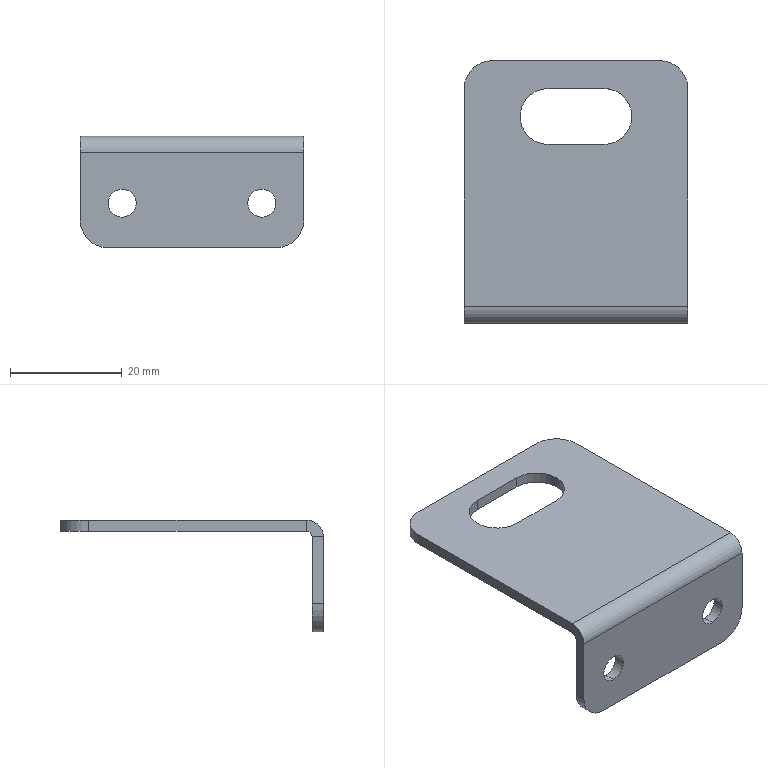Part | SolidWorks | features BaseBody 1 | 1 solid | 27 faces | box 40 x 47 x 20 mm | volume 4653 mm3 | plane 14 | cylinder 13 | commonest cylinder face diameters 10 x7 5 x4 2 x1 6 x1
STEP:
#1=CARTESIAN_POINT('',(-20.,-23.5,-15.));
#2=VERTEX_POINT('',#1);
#3=CARTESIAN_POINT('',(-15.,-23.5,-20.));
#4=VERTEX_POINT('',#3);
#5=CARTESIAN_POINT('',(-15.,-23.5,-15.));
#6=DIRECTION('',(0.,-1.,0.));
#7=DIRECTION('',(0.,0.,1.));
#8=AXIS2_PLACEMENT_3D('',#5,#6,#7);
#9=CIRCLE('',#8,5.);
#10=EDGE_CURVE('',#2,#4,#9,.T.);
#11=ORIENTED_EDGE('',*,*,#10,.F.);
#12=CARTESIAN_POINT('',(-20.,-21.5,-15.));
#13=VERTEX_POINT('',#12);
#14=CARTESIAN_POINT('',(-20.,-23.5,-15.));
#15=DIRECTION('',(0.,-1.,0.));
#16=VECTOR('',#15,1000.);
#17=LINE('',#14,#16);
#18=EDGE_CURVE('',#13,#2,#17,.T.);
#19=ORIENTED_EDGE('',*,*,#18,.F.);
#20=CARTESIAN_POINT('',(-15.,-21.5,-20.));
#21=VERTEX_POINT('',#20);
#22=CARTESIAN_POINT('',(-15.,-21.5,-15.));
#23=DIRECTION('',(0.,1.,0.));
#24=DIRECTION('',(0.,0.,1.));
#25=AXIS2_PLACEMENT_3D('',#22,#23,#24);
#26=CIRCLE('',#25,5.);
#27=EDGE_CURVE('',#21,#13,#26,.T.);
#28=ORIENTED_EDGE('',*,*,#27,.F.);
#29=CARTESIAN_POINT('',(-15.,-23.5,-20.));
#30=DIRECTION('',(0.,1.,0.));
#31=VECTOR('',#30,1000.);
#32=LINE('',#29,#31);
#33=EDGE_CURVE('',#4,#21,#32,.T.);
#34=ORIENTED_EDGE('',*,*,#33,.F.);
#35=EDGE_LOOP('',(#11,#19,#28,#34));
#36=FACE_OUTER_BOUND('',#35,.T.);
#37=CARTESIAN_POINT('',(-15.,-23.5,-15.));
#38=DIRECTION('',(0.,1.,0.));
#39=DIRECTION('',(0.,0.,1.));
#40=AXIS2_PLACEMENT_3D('',#37,#38,#39);
#41=CYLINDRICAL_SURFACE('',#40,5.);
#42=ADVANCED_FACE('',(#36),#41,.T.);
#43=CARTESIAN_POINT('',(15.,-23.5,-20.));
#44=VERTEX_POINT('',#43);
#45=CARTESIAN_POINT('',(20.,-23.5,-15.));
#46=VERTEX_POINT('',#45);
#47=CARTESIAN_POINT('',(15.,-23.5,-15.));
#48=DIRECTION('',(0.,-1.,0.));
#49=DIRECTION('',(0.,0.,1.));
#50=AXIS2_PLACEMENT_3D('',#47,#48,#49);
#51=CIRCLE('',#50,5.);
#52=EDGE_CURVE('',#44,#46,#51,.T.);
#53=ORIENTED_EDGE('',*,*,#52,.F.);
#54=CARTESIAN_POINT('',(15.,-21.5,-20.));
#55=VERTEX_POINT('',#54);
#56=CARTESIAN_POINT('',(15.,-23.5,-20.));
#57=DIRECTION('',(0.,-1.,0.));
#58=VECTOR('',#57,1000.);
#59=LINE('',#56,#58);
#60=EDGE_CURVE('',#55,#44,#59,.T.);
#61=ORIENTED_EDGE('',*,*,#60,.F.);
#62=CARTESIAN_POINT('',(20.,-21.5,-15.));
#63=VERTEX_POINT('',#62);
#64=CARTESIAN_POINT('',(15.,-21.5,-15.));
#65=DIRECTION('',(0.,1.,0.));
#66=DIRECTION('',(0.,0.,1.));
#67=AXIS2_PLACEMENT_3D('',#64,#65,#66);
#68=CIRCLE('',#67,5.);
#69=EDGE_CURVE('',#63,#55,#68,.T.);
#70=ORIENTED_EDGE('',*,*,#69,.F.);
#71=CARTESIAN_POINT('',(20.,-23.5,-15.));
#72=DIRECTION('',(0.,1.,0.));
#73=VECTOR('',#72,1000.);
#74=LINE('',#71,#73);
#75=EDGE_CURVE('',#46,#63,#74,.T.);
#76=ORIENTED_EDGE('',*,*,#75,.F.);
#77=EDGE_LOOP('',(#53,#61,#70,#76));
#78=FACE_OUTER_BOUND('',#77,.T.);
#79=CARTESIAN_POINT('',(15.,-23.5,-15.));
#80=DIRECTION('',(0.,1.,0.));
#81=DIRECTION('',(0.,0.,1.));
#82=AXIS2_PLACEMENT_3D('',#79,#80,#81);
#83=CYLINDRICAL_SURFACE('',#82,5.);
#84=ADVANCED_FACE('',(#78),#83,.T.);
#85=CARTESIAN_POINT('',(15.,23.5,-2.));
#86=VERTEX_POINT('',#85);
#87=CARTESIAN_POINT('',(20.,18.5,-2.));
#88=VERTEX_POINT('',#87);
#89=CARTESIAN_POINT('',(15.,18.5,-2.));
#90=DIRECTION('',(0.,0.,-1.));
#91=DIRECTION('',(-1.,0.,0.));
#92=AXIS2_PLACEMENT_3D('',#89,#90,#91);
#93=CIRCLE('',#92,5.);
#94=EDGE_CURVE('',#86,#88,#93,.T.);
#95=ORIENTED_EDGE('',*,*,#94,.F.);
#96=CARTESIAN_POINT('',(15.,23.5,0.));
#97=VERTEX_POINT('',#96);
#98=CARTESIAN_POINT('',(15.,23.5,-2.));
#99=DIRECTION('',(0.,0.,-1.));
#100=VECTOR('',#99,1000.);
#101=LINE('',#98,#100);
#102=EDGE_CURVE('',#97,#86,#101,.T.);
#103=ORIENTED_EDGE('',*,*,#102,.F.);
#104=CARTESIAN_POINT('',(20.,18.5,0.));
#105=VERTEX_POINT('',#104);
#106=CARTESIAN_POINT('',(15.,18.5,0.));
#107=DIRECTION('',(0.,0.,1.));
#108=DIRECTION('',(-1.,0.,0.));
#109=AXIS2_PLACEMENT_3D('',#106,#107,#108);
#110=CIRCLE('',#109,5.);
#111=EDGE_CURVE('',#105,#97,#110,.T.);
#112=ORIENTED_EDGE('',*,*,#111,.F.);
#113=CARTESIAN_POINT('',(20.,18.5,-2.));
#114=DIRECTION('',(0.,0.,1.));
#115=VECTOR('',#114,1000.);
#116=LINE('',#113,#115);
#117=EDGE_CURVE('',#88,#105,#116,.T.);
#118=ORIENTED_EDGE('',*,*,#117,.F.);
#119=EDGE_LOOP('',(#95,#103,#112,#118));
#120=FACE_OUTER_BOUND('',#119,.T.);
#121=CARTESIAN_POINT('',(15.,18.5,-2.));
#122=DIRECTION('',(0.,0.,1.));
#123=DIRECTION('',(1.,0.,0.));
#124=AXIS2_PLACEMENT_3D('',#121,#122,#123);
#125=CYLINDRICAL_SURFACE('',#124,5.);
#126=ADVANCED_FACE('',(#120),#125,.T.);
#127=CARTESIAN_POINT('',(-20.,18.5,-2.));
#128=VERTEX_POINT('',#127);
#129=CARTESIAN_POINT('',(-15.,23.5,-2.));
#130=VERTEX_POINT('',#129);
#131=CARTESIAN_POINT('',(-15.,18.5,-2.));
#132=DIRECTION('',(0.,0.,-1.));
#133=DIRECTION('',(-1.,0.,0.));
#134=AXIS2_PLACEMENT_3D('',#131,#132,#133);
#135=CIRCLE('',#134,5.);
#136=EDGE_CURVE('',#128,#130,#135,.T.);
#137=ORIENTED_EDGE('',*,*,#136,.F.);
#138=CARTESIAN_POINT('',(-20.,18.5,0.));
#139=VERTEX_POINT('',#138);
#140=CARTESIAN_POINT('',(-20.,18.5,-2.));
#141=DIRECTION('',(0.,0.,-1.));
#142=VECTOR('',#141,1000.);
#143=LINE('',#140,#142);
#144=EDGE_CURVE('',#139,#128,#143,.T.);
#145=ORIENTED_EDGE('',*,*,#144,.F.);
#146=CARTESIAN_POINT('',(-15.,23.5,0.));
#147=VERTEX_POINT('',#146);
#148=CARTESIAN_POINT('',(-15.,18.5,0.));
#149=DIRECTION('',(0.,0.,1.));
#150=DIRECTION('',(-1.,0.,0.));
#151=AXIS2_PLACEMENT_3D('',#148,#149,#150);
#152=CIRCLE('',#151,5.);
#153=EDGE_CURVE('',#147,#139,#152,.T.);
#154=ORIENTED_EDGE('',*,*,#153,.F.);
#155=CARTESIAN_POINT('',(-15.,23.5,-2.));
#156=DIRECTION('',(0.,0.,1.));
#157=VECTOR('',#156,1000.);
#158=LINE('',#155,#157);
#159=EDGE_CURVE('',#130,#147,#158,.T.);
#160=ORIENTED_EDGE('',*,*,#159,.F.);
#161=EDGE_LOOP('',(#137,#145,#154,#160));
#162=FACE_OUTER_BOUND('',#161,.T.);
#163=CARTESIAN_POINT('',(-15.,18.5,-2.));
#164=DIRECTION('',(0.,0.,1.));
#165=DIRECTION('',(1.,0.,0.));
#166=AXIS2_PLACEMENT_3D('',#163,#164,#165);
#167=CYLINDRICAL_SURFACE('',#166,5.);
#168=ADVANCED_FACE('',(#162),#167,.T.);
#169=CARTESIAN_POINT('',(-12.5,-21.5,-9.5));
#170=VERTEX_POINT('',#169);
#171=CARTESIAN_POINT('',(-12.5,-23.5,-9.5));
#172=VERTEX_POINT('',#171);
#173=CARTESIAN_POINT('',(-12.5,-21.5,-9.5));
#174=DIRECTION('',(0.,-1.,0.));
#175=VECTOR('',#174,1000.);
#176=LINE('',#173,#175);
#177=EDGE_CURVE('',#170,#172,#176,.T.);
#178=ORIENTED_EDGE('',*,*,#177,.F.);
#179=CARTESIAN_POINT('',(-12.5,-21.5,-14.5));
#180=VERTEX_POINT('',#179);
#181=CARTESIAN_POINT('',(-12.5,-21.5,-12.));
#182=DIRECTION('',(0.,-1.,0.));
#183=DIRECTION('',(0.,0.,-1.));
#184=AXIS2_PLACEMENT_3D('',#181,#182,#183);
#185=CIRCLE('',#184,2.5);
#186=EDGE_CURVE('',#180,#170,#185,.T.);
#187=ORIENTED_EDGE('',*,*,#186,.F.);
#188=CARTESIAN_POINT('',(-12.5,-23.5,-14.5));
#189=VERTEX_POINT('',#188);
#190=CARTESIAN_POINT('',(-12.5,-21.5,-14.5));
#191=DIRECTION('',(0.,-1.,0.));
#192=VECTOR('',#191,1000.);
#193=LINE('',#190,#192);
#194=EDGE_CURVE('',#180,#189,#193,.T.);
#195=ORIENTED_EDGE('',*,*,#194,.T.);
#196=CARTESIAN_POINT('',(-12.5,-23.5,-12.));
#197=DIRECTION('',(0.,-1.,0.));
#198=DIRECTION('',(0.,0.,-1.));
#199=AXIS2_PLACEMENT_3D('',#196,#197,#198);
#200=CIRCLE('',#199,2.5);
#201=EDGE_CURVE('',#189,#172,#200,.T.);
#202=ORIENTED_EDGE('',*,*,#201,.T.);
#203=EDGE_LOOP('',(#178,#187,#195,#202));
#204=FACE_OUTER_BOUND('',#203,.T.);
#205=CARTESIAN_POINT('',(-12.5,-21.5,-12.));
#206=DIRECTION('',(0.,-1.,0.));
#207=DIRECTION('',(0.,0.,-1.));
#208=AXIS2_PLACEMENT_3D('',#205,#206,#207);
#209=CYLINDRICAL_SURFACE('',#208,2.5);
#210=ADVANCED_FACE('',(#204),#209,.F.);
#211=CARTESIAN_POINT('',(12.5,-21.5,-9.5));
#212=VERTEX_POINT('',#211);
#213=CARTESIAN_POINT('',(12.5,-23.5,-9.5));
#214=VERTEX_POINT('',#213);
#215=CARTESIAN_POINT('',(12.5,-21.5,-9.5));
#216=DIRECTION('',(0.,-1.,0.));
#217=VECTOR('',#216,1000.);
#218=LINE('',#215,#217);
#219=EDGE_CURVE('',#212,#214,#218,.T.);
#220=ORIENTED_EDGE('',*,*,#219,.F.);
#221=CARTESIAN_POINT('',(12.5,-21.5,-14.5));
#222=VERTEX_POINT('',#221);
#223=CARTESIAN_POINT('',(12.5,-21.5,-12.));
#224=DIRECTION('',(0.,-1.,0.));
#225=DIRECTION('',(0.,0.,1.));
#226=AXIS2_PLACEMENT_3D('',#223,#224,#225);
#227=CIRCLE('',#226,2.5);
#228=EDGE_CURVE('',#222,#212,#227,.T.);
#229=ORIENTED_EDGE('',*,*,#228,.F.);
#230=CARTESIAN_POINT('',(12.5,-23.5,-14.5));
#231=VERTEX_POINT('',#230);
#232=CARTESIAN_POINT('',(12.5,-21.5,-14.5));
#233=DIRECTION('',(0.,-1.,0.));
#234=VECTOR('',#233,1000.);
#235=LINE('',#232,#234);
#236=EDGE_CURVE('',#222,#231,#235,.T.);
#237=ORIENTED_EDGE('',*,*,#236,.T.);
#238=CARTESIAN_POINT('',(12.5,-23.5,-12.));
#239=DIRECTION('',(0.,-1.,0.));
#240=DIRECTION('',(0.,0.,1.));
#241=AXIS2_PLACEMENT_3D('',#238,#239,#240);
#242=CIRCLE('',#241,2.5);
#243=EDGE_CURVE('',#231,#214,#242,.T.);
#244=ORIENTED_EDGE('',*,*,#243,.T.);
#245=EDGE_LOOP('',(#220,#229,#237,#244));
#246=FACE_OUTER_BOUND('',#245,.T.);
#247=CARTESIAN_POINT('',(12.5,-21.5,-12.));
#248=DIRECTION('',(0.,-1.,0.));
#249=DIRECTION('',(0.,0.,-1.));
#250=AXIS2_PLACEMENT_3D('',#247,#248,#249);
#251=CYLINDRICAL_SURFACE('',#250,2.5);
#252=ADVANCED_FACE('',(#246),#251,.F.);
#253=CARTESIAN_POINT('',(5.,18.5,0.));
#254=VERTEX_POINT('',#253);
#255=CARTESIAN_POINT('',(-5.,18.5,0.));
#256=VERTEX_POINT('',#255);
#257=CARTESIAN_POINT('',(5.,18.5,0.));
#258=DIRECTION('',(-1.,0.,0.));
#259=VECTOR('',#258,1000.);
#260=LINE('',#257,#259);
#261=EDGE_CURVE('',#254,#256,#260,.T.);
#262=ORIENTED_EDGE('',*,*,#261,.T.);
#263=CARTESIAN_POINT('',(-5.,18.5,-2.));
#264=VERTEX_POINT('',#263);
#265=CARTESIAN_POINT('',(-5.,18.5,-2.));
#266=DIRECTION('',(0.,0.,1.));
#267=VECTOR('',#266,1000.);
#268=LINE('',#265,#267);
#269=EDGE_CURVE('',#264,#256,#268,.T.);
#270=ORIENTED_EDGE('',*,*,#269,.F.);
#271=CARTESIAN_POINT('',(5.,18.5,-2.));
#272=VERTEX_POINT('',#271);
#273=CARTESIAN_POINT('',(5.,18.5,-2.));
#274=DIRECTION('',(-1.,0.,0.));
#275=VECTOR('',#274,1000.);
#276=LINE('',#273,#275);
#277=EDGE_CURVE('',#272,#264,#276,.T.);
#278=ORIENTED_EDGE('',*,*,#277,.F.);
#279=CARTESIAN_POINT('',(5.,18.5,-2.));
#280=DIRECTION('',(0.,0.,1.));
#281=VECTOR('',#280,1000.);
#282=LINE('',#279,#281);
#283=EDGE_CURVE('',#272,#254,#282,.T.);
#284=ORIENTED_EDGE('',*,*,#283,.T.);
#285=EDGE_LOOP('',(#262,#270,#278,#284));
#286=FACE_OUTER_BOUND('',#285,.T.);
#287=CARTESIAN_POINT('',(5.,18.5,-2.));
#288=DIRECTION('',(0.,1.,0.));
#289=DIRECTION('',(1.,0.,0.));
#290=AXIS2_PLACEMENT_3D('',#287,#288,#289);
#291=PLANE('',#290);
#292=ADVANCED_FACE('',(#286),#291,.F.);
#293=CARTESIAN_POINT('',(-5.,8.5,0.));
#294=VERTEX_POINT('',#293);
#295=CARTESIAN_POINT('',(-5.,13.5,0.));
#296=DIRECTION('',(0.,0.,1.));
#297=DIRECTION('',(1.,0.,0.));
#298=AXIS2_PLACEMENT_3D('',#295,#296,#297);
#299=CIRCLE('',#298,5.);
#300=EDGE_CURVE('',#256,#294,#299,.T.);
#301=ORIENTED_EDGE('',*,*,#300,.T.);
#302=CARTESIAN_POINT('',(-5.,8.5,-2.));
#303=VERTEX_POINT('',#302);
#304=CARTESIAN_POINT('',(-5.,8.5,-2.));
#305=DIRECTION('',(0.,0.,1.));
#306=VECTOR('',#305,1000.);
#307=LINE('',#304,#306);
#308=EDGE_CURVE('',#303,#294,#307,.T.);
#309=ORIENTED_EDGE('',*,*,#308,.F.);
#310=CARTESIAN_POINT('',(-5.,13.5,-2.));
#311=DIRECTION('',(0.,0.,1.));
#312=DIRECTION('',(1.,0.,0.));
#313=AXIS2_PLACEMENT_3D('',#310,#311,#312);
#314=CIRCLE('',#313,5.);
#315=EDGE_CURVE('',#264,#303,#314,.T.);
#316=ORIENTED_EDGE('',*,*,#315,.F.);
#317=ORIENTED_EDGE('',*,*,#269,.T.);
#318=EDGE_LOOP('',(#301,#309,#316,#317));
#319=FACE_OUTER_BOUND('',#318,.T.);
#320=CARTESIAN_POINT('',(-5.,13.5,-2.));
#321=DIRECTION('',(0.,0.,1.));
#322=DIRECTION('',(1.,0.,0.));
#323=AXIS2_PLACEMENT_3D('',#320,#321,#322);
#324=CYLINDRICAL_SURFACE('',#323,5.);
#325=ADVANCED_FACE('',(#319),#324,.F.);
#326=CARTESIAN_POINT('',(5.,8.5,0.));
#327=VERTEX_POINT('',#326);
#328=CARTESIAN_POINT('',(5.,8.5,0.));
#329=DIRECTION('',(1.,0.,0.));
#330=VECTOR('',#329,1000.);
#331=LINE('',#328,#330);
#332=EDGE_CURVE('',#294,#327,#331,.T.);
#333=ORIENTED_EDGE('',*,*,#332,.T.);
#334=CARTESIAN_POINT('',(5.,8.5,-2.));
#335=VERTEX_POINT('',#334);
#336=CARTESIAN_POINT('',(5.,8.5,-2.));
#337=DIRECTION('',(0.,0.,1.));
#338=VECTOR('',#337,1000.);
#339=LINE('',#336,#338);
#340=EDGE_CURVE('',#335,#327,#339,.T.);
#341=ORIENTED_EDGE('',*,*,#340,.F.);
#342=CARTESIAN_POINT('',(5.,8.5,-2.));
#343=DIRECTION('',(1.,0.,0.));
#344=VECTOR('',#343,1000.);
#345=LINE('',#342,#344);
#346=EDGE_CURVE('',#303,#335,#345,.T.);
#347=ORIENTED_EDGE('',*,*,#346,.F.);
#348=ORIENTED_EDGE('',*,*,#308,.T.);
#349=EDGE_LOOP('',(#333,#341,#347,#348));
#350=FACE_OUTER_BOUND('',#349,.T.);
#351=CARTESIAN_POINT('',(5.,8.5,-2.));
#352=DIRECTION('',(0.,-1.,0.));
#353=DIRECTION('',(-1.,0.,0.));
#354=AXIS2_PLACEMENT_3D('',#351,#352,#353);
#355=PLANE('',#354);
#356=ADVANCED_FACE('',(#350),#355,.F.);
#357=CARTESIAN_POINT('',(10.,13.5,-2.));
#358=VERTEX_POINT('',#357);
#359=CARTESIAN_POINT('',(10.,13.5,0.));
#360=VERTEX_POINT('',#359);
#361=CARTESIAN_POINT('',(10.,13.5,-2.));
#362=DIRECTION('',(0.,0.,1.));
#363=VECTOR('',#362,1000.);
#364=LINE('',#361,#363);
#365=EDGE_CURVE('',#358,#360,#364,.T.);
#366=ORIENTED_EDGE('',*,*,#365,.F.);
#367=CARTESIAN_POINT('',(5.,13.5,-2.));
#368=DIRECTION('',(0.,0.,1.));
#369=DIRECTION('',(1.,0.,0.));
#370=AXIS2_PLACEMENT_3D('',#367,#368,#369);
#371=CIRCLE('',#370,5.);
#372=EDGE_CURVE('',#335,#358,#371,.T.);
#373=ORIENTED_EDGE('',*,*,#372,.F.);
#374=ORIENTED_EDGE('',*,*,#340,.T.);
#375=CARTESIAN_POINT('',(5.,13.5,0.));
#376=DIRECTION('',(0.,0.,1.));
#377=DIRECTION('',(1.,0.,0.));
#378=AXIS2_PLACEMENT_3D('',#375,#376,#377);
#379=CIRCLE('',#378,5.);
#380=EDGE_CURVE('',#327,#360,#379,.T.);
#381=ORIENTED_EDGE('',*,*,#380,.T.);
#382=EDGE_LOOP('',(#366,#373,#374,#381));
#383=FACE_OUTER_BOUND('',#382,.T.);
#384=CARTESIAN_POINT('',(5.,13.5,-2.));
#385=DIRECTION('',(0.,0.,1.));
#386=DIRECTION('',(1.,0.,0.));
#387=AXIS2_PLACEMENT_3D('',#384,#385,#386);
#388=CYLINDRICAL_SURFACE('',#387,5.);
#389=ADVANCED_FACE('',(#383),#388,.F.);
#390=CARTESIAN_POINT('',(20.,-21.5,-20.));
#391=DIRECTION('',(1.,0.,0.));
#392=VECTOR('',#391,1000.);
#393=LINE('',#390,#392);
#394=EDGE_CURVE('',#21,#55,#393,.T.);
#395=ORIENTED_EDGE('',*,*,#394,.T.);
#396=ORIENTED_EDGE('',*,*,#60,.T.);
#397=CARTESIAN_POINT('',(0.,-23.5,-20.));
#398=DIRECTION('',(1.,0.,0.));
#399=VECTOR('',#398,1000.);
#400=LINE('',#397,#399);
#401=EDGE_CURVE('',#4,#44,#400,.T.);
#402=ORIENTED_EDGE('',*,*,#401,.F.);
#403=ORIENTED_EDGE('',*,*,#33,.T.);
#404=EDGE_LOOP('',(#395,#396,#402,#403));
#405=FACE_OUTER_BOUND('',#404,.T.);
#406=CARTESIAN_POINT('',(20.,-23.5,-20.));
#407=DIRECTION('',(0.,0.,1.));
#408=DIRECTION('',(0.,-1.,0.));
#409=AXIS2_PLACEMENT_3D('',#406,#407,#408);
#410=PLANE('',#409);
#411=ADVANCED_FACE('',(#405),#410,.F.);
#412=ORIENTED_EDGE('',*,*,#228,.T.);
#413=CARTESIAN_POINT('',(12.5,-21.5,-12.));
#414=DIRECTION('',(0.,-1.,0.));
#415=DIRECTION('',(0.,0.,1.));
#416=AXIS2_PLACEMENT_3D('',#413,#414,#415);
#417=CIRCLE('',#416,2.5);
#418=EDGE_CURVE('',#212,#222,#417,.T.);
#419=ORIENTED_EDGE('',*,*,#418,.T.);
#420=EDGE_LOOP('',(#412,#419));
#421=FACE_BOUND('',#420,.T.);
#422=ORIENTED_EDGE('',*,*,#186,.T.);
#423=CARTESIAN_POINT('',(-12.5,-21.5,-12.));
#424=DIRECTION('',(0.,-1.,0.));
#425=DIRECTION('',(0.,0.,-1.));
#426=AXIS2_PLACEMENT_3D('',#423,#424,#425);
#427=CIRCLE('',#426,2.5);
#428=EDGE_CURVE('',#170,#180,#427,.T.);
#429=ORIENTED_EDGE('',*,*,#428,.T.);
#430=EDGE_LOOP('',(#422,#429));
#431=FACE_BOUND('',#430,.T.);
#432=CARTESIAN_POINT('',(20.,-21.5,-3.));
#433=VERTEX_POINT('',#432);
#434=CARTESIAN_POINT('',(20.,-21.5,-2.));
#435=DIRECTION('',(0.,0.,1.));
#436=VECTOR('',#435,1000.);
#437=LINE('',#434,#436);
#438=EDGE_CURVE('',#63,#433,#437,.T.);
#439=ORIENTED_EDGE('',*,*,#438,.F.);
#440=ORIENTED_EDGE('',*,*,#69,.T.);
#441=ORIENTED_EDGE('',*,*,#394,.F.);
#442=ORIENTED_EDGE('',*,*,#27,.T.);
#443=CARTESIAN_POINT('',(-20.,-21.5,-3.));
#444=VERTEX_POINT('',#443);
#445=CARTESIAN_POINT('',(-20.,-21.5,-20.));
#446=DIRECTION('',(0.,0.,-1.));
#447=VECTOR('',#446,1000.);
#448=LINE('',#445,#447);
#449=EDGE_CURVE('',#444,#13,#448,.T.);
#450=ORIENTED_EDGE('',*,*,#449,.F.);
#451=CARTESIAN_POINT('',(20.,-21.5,-3.));
#452=DIRECTION('',(-1.,0.,0.));
#453=VECTOR('',#452,1000.);
#454=LINE('',#451,#453);
#455=EDGE_CURVE('',#433,#444,#454,.T.);
#456=ORIENTED_EDGE('',*,*,#455,.F.);
#457=EDGE_LOOP('',(#439,#440,#441,#442,#450,#456));
#458=FACE_OUTER_BOUND('',#457,.T.);
#459=CARTESIAN_POINT('',(0.,-21.5,0.));
#460=DIRECTION('',(0.,1.,0.));
#461=DIRECTION('',(0.,0.,-1.));
#462=AXIS2_PLACEMENT_3D('',#459,#460,#461);
#463=PLANE('',#462);
#464=ADVANCED_FACE('',(#421,#431,#458),#463,.T.);
#465=ORIENTED_EDGE('',*,*,#243,.F.);
#466=CARTESIAN_POINT('',(12.5,-23.5,-12.));
#467=DIRECTION('',(0.,-1.,0.));
#468=DIRECTION('',(0.,0.,1.));
#469=AXIS2_PLACEMENT_3D('',#466,#467,#468);
#470=CIRCLE('',#469,2.5);
#471=EDGE_CURVE('',#214,#231,#470,.T.);
#472=ORIENTED_EDGE('',*,*,#471,.F.);
#473=EDGE_LOOP('',(#465,#472));
#474=FACE_BOUND('',#473,.T.);
#475=ORIENTED_EDGE('',*,*,#201,.F.);
#476=CARTESIAN_POINT('',(-12.5,-23.5,-12.));
#477=DIRECTION('',(0.,-1.,0.));
#478=DIRECTION('',(0.,0.,-1.));
#479=AXIS2_PLACEMENT_3D('',#476,#477,#478);
#480=CIRCLE('',#479,2.5);
#481=EDGE_CURVE('',#172,#189,#480,.T.);
#482=ORIENTED_EDGE('',*,*,#481,.F.);
#483=EDGE_LOOP('',(#475,#482));
#484=FACE_BOUND('',#483,.T.);
#485=ORIENTED_EDGE('',*,*,#401,.T.);
#486=ORIENTED_EDGE('',*,*,#52,.T.);
#487=CARTESIAN_POINT('',(20.,-23.5,-3.));
#488=VERTEX_POINT('',#487);
#489=CARTESIAN_POINT('',(20.,-23.5,0.));
#490=DIRECTION('',(0.,0.,1.));
#491=VECTOR('',#490,1000.);
#492=LINE('',#489,#491);
#493=EDGE_CURVE('',#46,#488,#492,.T.);
#494=ORIENTED_EDGE('',*,*,#493,.T.);
#495=CARTESIAN_POINT('',(-20.,-23.5,-3.));
#496=VERTEX_POINT('',#495);
#497=CARTESIAN_POINT('',(20.,-23.5,-3.));
#498=DIRECTION('',(1.,0.,0.));
#499=VECTOR('',#498,1000.);
#500=LINE('',#497,#499);
#501=EDGE_CURVE('',#496,#488,#500,.T.);
#502=ORIENTED_EDGE('',*,*,#501,.F.);
#503=CARTESIAN_POINT('',(-20.,-23.5,0.));
#504=DIRECTION('',(0.,0.,-1.));
#505=VECTOR('',#504,1000.);
#506=LINE('',#503,#505);
#507=EDGE_CURVE('',#496,#2,#506,.T.);
#508=ORIENTED_EDGE('',*,*,#507,.T.);
#509=ORIENTED_EDGE('',*,*,#10,.T.);
#510=EDGE_LOOP('',(#485,#486,#494,#502,#508,#509));
#511=FACE_OUTER_BOUND('',#510,.T.);
#512=CARTESIAN_POINT('',(0.,-23.5,0.));
#513=DIRECTION('',(0.,1.,0.));
#514=DIRECTION('',(0.,0.,-1.));
#515=AXIS2_PLACEMENT_3D('',#512,#513,#514);
#516=PLANE('',#515);
#517=ADVANCED_FACE('',(#474,#484,#511),#516,.F.);
#518=ORIENTED_EDGE('',*,*,#493,.F.);
#519=ORIENTED_EDGE('',*,*,#75,.T.);
#520=ORIENTED_EDGE('',*,*,#438,.T.);
#521=CARTESIAN_POINT('',(20.,-23.5,-3.));
#522=DIRECTION('',(0.,-1.,0.));
#523=VECTOR('',#522,1000.);
#524=LINE('',#521,#523);
#525=EDGE_CURVE('',#433,#488,#524,.T.);
#526=ORIENTED_EDGE('',*,*,#525,.T.);
#527=EDGE_LOOP('',(#518,#519,#520,#526));
#528=FACE_OUTER_BOUND('',#527,.T.);
#529=CARTESIAN_POINT('',(20.,-23.5,-2.));
#530=DIRECTION('',(-1.,0.,0.));
#531=DIRECTION('',(0.,1.,0.));
#532=AXIS2_PLACEMENT_3D('',#529,#530,#531);
#533=PLANE('',#532);
#534=ADVANCED_FACE('',(#528),#533,.F.);
#535=ORIENTED_EDGE('',*,*,#449,.T.);
#536=ORIENTED_EDGE('',*,*,#18,.T.);
#537=ORIENTED_EDGE('',*,*,#507,.F.);
#538=CARTESIAN_POINT('',(-20.,-21.5,-3.));
#539=DIRECTION('',(0.,-1.,0.));
#540=VECTOR('',#539,1000.);
#541=LINE('',#538,#540);
#542=EDGE_CURVE('',#444,#496,#541,.T.);
#543=ORIENTED_EDGE('',*,*,#542,.F.);
#544=EDGE_LOOP('',(#535,#536,#537,#543));
#545=FACE_OUTER_BOUND('',#544,.T.);
#546=CARTESIAN_POINT('',(-20.,-23.5,-20.));
#547=DIRECTION('',(1.,0.,0.));
#548=DIRECTION('',(0.,1.,0.));
#549=AXIS2_PLACEMENT_3D('',#546,#547,#548);
#550=PLANE('',#549);
#551=ADVANCED_FACE('',(#545),#550,.F.);
#552=CARTESIAN_POINT('',(-20.,-20.5,-2.));
#553=VERTEX_POINT('',#552);
#554=CARTESIAN_POINT('',(20.,-20.5,-2.));
#555=VERTEX_POINT('',#554);
#556=CARTESIAN_POINT('',(-20.,-20.5,-2.));
#557=DIRECTION('',(1.,0.,0.));
#558=VECTOR('',#557,1000.);
#559=LINE('',#556,#558);
#560=EDGE_CURVE('',#553,#555,#559,.T.);
#561=ORIENTED_EDGE('',*,*,#560,.T.);
#562=CARTESIAN_POINT('',(20.,-20.5,-3.));
#563=DIRECTION('',(1.,0.,0.));
#564=DIRECTION('',(0.,0.,1.));
#565=AXIS2_PLACEMENT_3D('',#562,#563,#564);
#566=CIRCLE('',#565,1.);
#567=EDGE_CURVE('',#555,#433,#566,.T.);
#568=ORIENTED_EDGE('',*,*,#567,.T.);
#569=ORIENTED_EDGE('',*,*,#455,.T.);
#570=CARTESIAN_POINT('',(-20.,-20.5,-3.));
#571=DIRECTION('',(-1.,0.,0.));
#572=DIRECTION('',(0.,0.,1.));
#573=AXIS2_PLACEMENT_3D('',#570,#571,#572);
#574=CIRCLE('',#573,1.);
#575=EDGE_CURVE('',#444,#553,#574,.T.);
#576=ORIENTED_EDGE('',*,*,#575,.T.);
#577=EDGE_LOOP('',(#561,#568,#569,#576));
#578=FACE_OUTER_BOUND('',#577,.T.);
#579=CARTESIAN_POINT('',(-20.,-20.5,-3.));
#580=DIRECTION('',(-1.,0.,0.));
#581=DIRECTION('',(0.,-1.,0.));
#582=AXIS2_PLACEMENT_3D('',#579,#580,#581);
#583=CYLINDRICAL_SURFACE('',#582,1.);
#584=ADVANCED_FACE('',(#578),#583,.F.);
#585=CARTESIAN_POINT('',(-20.,-20.5,0.));
#586=VERTEX_POINT('',#585);
#587=CARTESIAN_POINT('',(20.,-20.5,0.));
#588=VERTEX_POINT('',#587);
#589=CARTESIAN_POINT('',(-20.,-20.5,0.));
#590=DIRECTION('',(1.,0.,0.));
#591=VECTOR('',#590,1000.);
#592=LINE('',#589,#591);
#593=EDGE_CURVE('',#586,#588,#592,.T.);
#594=ORIENTED_EDGE('',*,*,#593,.F.);
#595=CARTESIAN_POINT('',(-20.,-20.5,-3.));
#596=DIRECTION('',(-1.,0.,0.));
#597=DIRECTION('',(0.,0.,1.));
#598=AXIS2_PLACEMENT_3D('',#595,#596,#597);
#599=CIRCLE('',#598,3.);
#600=EDGE_CURVE('',#496,#586,#599,.T.);
#601=ORIENTED_EDGE('',*,*,#600,.F.);
#602=ORIENTED_EDGE('',*,*,#501,.T.);
#603=CARTESIAN_POINT('',(20.,-20.5,-3.));
#604=DIRECTION('',(1.,0.,0.));
#605=DIRECTION('',(0.,0.,1.));
#606=AXIS2_PLACEMENT_3D('',#603,#604,#605);
#607=CIRCLE('',#606,3.);
#608=EDGE_CURVE('',#588,#488,#607,.T.);
#609=ORIENTED_EDGE('',*,*,#608,.F.);
#610=EDGE_LOOP('',(#594,#601,#602,#609));
#611=FACE_OUTER_BOUND('',#610,.T.);
#612=CARTESIAN_POINT('',(-20.,-20.5,-3.));
#613=DIRECTION('',(-1.,0.,0.));
#614=DIRECTION('',(0.,-1.,0.));
#615=AXIS2_PLACEMENT_3D('',#612,#613,#614);
#616=CYLINDRICAL_SURFACE('',#615,3.);
#617=ADVANCED_FACE('',(#611),#616,.T.);
#618=ORIENTED_EDGE('',*,*,#575,.F.);
#619=ORIENTED_EDGE('',*,*,#542,.T.);
#620=ORIENTED_EDGE('',*,*,#600,.T.);
#621=CARTESIAN_POINT('',(-20.,-20.5,-2.));
#622=DIRECTION('',(0.,0.,1.));
#623=VECTOR('',#622,1000.);
#624=LINE('',#621,#623);
#625=EDGE_CURVE('',#553,#586,#624,.T.);
#626=ORIENTED_EDGE('',*,*,#625,.F.);
#627=EDGE_LOOP('',(#618,#619,#620,#626));
#628=FACE_OUTER_BOUND('',#627,.T.);
#629=CARTESIAN_POINT('',(-20.,-20.5,-3.));
#630=DIRECTION('',(1.,0.,0.));
#631=DIRECTION('',(0.,1.,0.));
#632=AXIS2_PLACEMENT_3D('',#629,#630,#631);
#633=PLANE('',#632);
#634=ADVANCED_FACE('',(#628),#633,.F.);
#635=ORIENTED_EDGE('',*,*,#525,.F.);
#636=ORIENTED_EDGE('',*,*,#567,.F.);
#637=CARTESIAN_POINT('',(20.,-20.5,-2.));
#638=DIRECTION('',(0.,0.,1.));
#639=VECTOR('',#638,1000.);
#640=LINE('',#637,#639);
#641=EDGE_CURVE('',#555,#588,#640,.T.);
#642=ORIENTED_EDGE('',*,*,#641,.T.);
#643=ORIENTED_EDGE('',*,*,#608,.T.);
#644=EDGE_LOOP('',(#635,#636,#642,#643));
#645=FACE_OUTER_BOUND('',#644,.T.);
#646=CARTESIAN_POINT('',(20.,-20.5,-3.));
#647=DIRECTION('',(1.,0.,0.));
#648=DIRECTION('',(0.,1.,0.));
#649=AXIS2_PLACEMENT_3D('',#646,#647,#648);
#650=PLANE('',#649);
#651=ADVANCED_FACE('',(#645),#650,.T.);
#652=CARTESIAN_POINT('',(20.,23.5,-2.));
#653=DIRECTION('',(0.,1.,0.));
#654=VECTOR('',#653,1000.);
#655=LINE('',#652,#654);
#656=EDGE_CURVE('',#555,#88,#655,.T.);
#657=ORIENTED_EDGE('',*,*,#656,.T.);
#658=ORIENTED_EDGE('',*,*,#117,.T.);
#659=CARTESIAN_POINT('',(20.,23.5,0.));
#660=DIRECTION('',(0.,1.,0.));
#661=VECTOR('',#660,1000.);
#662=LINE('',#659,#661);
#663=EDGE_CURVE('',#588,#105,#662,.T.);
#664=ORIENTED_EDGE('',*,*,#663,.F.);
#665=ORIENTED_EDGE('',*,*,#641,.F.);
#666=EDGE_LOOP('',(#657,#658,#664,#665));
#667=FACE_OUTER_BOUND('',#666,.T.);
#668=CARTESIAN_POINT('',(20.,23.5,-2.));
#669=DIRECTION('',(1.,0.,0.));
#670=DIRECTION('',(0.,1.,0.));
#671=AXIS2_PLACEMENT_3D('',#668,#669,#670);
#672=PLANE('',#671);
#673=ADVANCED_FACE('',(#667),#672,.T.);
#674=CARTESIAN_POINT('',(20.,23.5,-2.));
#675=DIRECTION('',(-1.,0.,0.));
#676=VECTOR('',#675,1000.);
#677=LINE('',#674,#676);
#678=EDGE_CURVE('',#86,#130,#677,.T.);
#679=ORIENTED_EDGE('',*,*,#678,.T.);
#680=ORIENTED_EDGE('',*,*,#159,.T.);
#681=CARTESIAN_POINT('',(20.,23.5,0.));
#682=DIRECTION('',(-1.,0.,0.));
#683=VECTOR('',#682,1000.);
#684=LINE('',#681,#683);
#685=EDGE_CURVE('',#97,#147,#684,.T.);
#686=ORIENTED_EDGE('',*,*,#685,.F.);
#687=ORIENTED_EDGE('',*,*,#102,.T.);
#688=EDGE_LOOP('',(#679,#680,#686,#687));
#689=FACE_OUTER_BOUND('',#688,.T.);
#690=CARTESIAN_POINT('',(20.,23.5,-2.));
#691=DIRECTION('',(0.,1.,0.));
#692=DIRECTION('',(1.,0.,0.));
#693=AXIS2_PLACEMENT_3D('',#690,#691,#692);
#694=PLANE('',#693);
#695=ADVANCED_FACE('',(#689),#694,.T.);
#696=ORIENTED_EDGE('',*,*,#261,.F.);
#697=CARTESIAN_POINT('',(5.,13.5,0.));
#698=DIRECTION('',(0.,0.,1.));
#699=DIRECTION('',(1.,0.,0.));
#700=AXIS2_PLACEMENT_3D('',#697,#698,#699);
#701=CIRCLE('',#700,5.);
#702=EDGE_CURVE('',#360,#254,#701,.T.);
#703=ORIENTED_EDGE('',*,*,#702,.F.);
#704=ORIENTED_EDGE('',*,*,#380,.F.);
#705=ORIENTED_EDGE('',*,*,#332,.F.);
#706=ORIENTED_EDGE('',*,*,#300,.F.);
#707=EDGE_LOOP('',(#696,#703,#704,#705,#706));
#708=FACE_BOUND('',#707,.T.);
#709=ORIENTED_EDGE('',*,*,#685,.T.);
#710=ORIENTED_EDGE('',*,*,#153,.T.);
#711=CARTESIAN_POINT('',(-20.,23.5,0.));
#712=DIRECTION('',(0.,-1.,0.));
#713=VECTOR('',#712,1000.);
#714=LINE('',#711,#713);
#715=EDGE_CURVE('',#139,#586,#714,.T.);
#716=ORIENTED_EDGE('',*,*,#715,.T.);
#717=ORIENTED_EDGE('',*,*,#593,.T.);
#718=ORIENTED_EDGE('',*,*,#663,.T.);
#719=ORIENTED_EDGE('',*,*,#111,.T.);
#720=EDGE_LOOP('',(#709,#710,#716,#717,#718,#719));
#721=FACE_OUTER_BOUND('',#720,.T.);
#722=CARTESIAN_POINT('',(0.,0.,0.));
#723=DIRECTION('',(0.,0.,-1.));
#724=DIRECTION('',(0.,-1.,0.));
#725=AXIS2_PLACEMENT_3D('',#722,#723,#724);
#726=PLANE('',#725);
#727=ADVANCED_FACE('',(#708,#721),#726,.F.);
#728=ORIENTED_EDGE('',*,*,#372,.T.);
#729=CARTESIAN_POINT('',(5.,13.5,-2.));
#730=DIRECTION('',(0.,0.,1.));
#731=DIRECTION('',(1.,0.,0.));
#732=AXIS2_PLACEMENT_3D('',#729,#730,#731);
#733=CIRCLE('',#732,5.);
#734=EDGE_CURVE('',#358,#272,#733,.T.);
#735=ORIENTED_EDGE('',*,*,#734,.T.);
#736=ORIENTED_EDGE('',*,*,#277,.T.);
#737=ORIENTED_EDGE('',*,*,#315,.T.);
#738=ORIENTED_EDGE('',*,*,#346,.T.);
#739=EDGE_LOOP('',(#728,#735,#736,#737,#738));
#740=FACE_BOUND('',#739,.T.);
#741=CARTESIAN_POINT('',(-20.,23.5,-2.));
#742=DIRECTION('',(0.,-1.,0.));
#743=VECTOR('',#742,1000.);
#744=LINE('',#741,#743);
#745=EDGE_CURVE('',#128,#553,#744,.T.);
#746=ORIENTED_EDGE('',*,*,#745,.F.);
#747=ORIENTED_EDGE('',*,*,#136,.T.);
#748=ORIENTED_EDGE('',*,*,#678,.F.);
#749=ORIENTED_EDGE('',*,*,#94,.T.);
#750=ORIENTED_EDGE('',*,*,#656,.F.);
#751=ORIENTED_EDGE('',*,*,#560,.F.);
#752=EDGE_LOOP('',(#746,#747,#748,#749,#750,#751));
#753=FACE_OUTER_BOUND('',#752,.T.);
#754=CARTESIAN_POINT('',(0.,0.,-2.));
#755=DIRECTION('',(0.,0.,-1.));
#756=DIRECTION('',(0.,-1.,0.));
#757=AXIS2_PLACEMENT_3D('',#754,#755,#756);
#758=PLANE('',#757);
#759=ADVANCED_FACE('',(#740,#753),#758,.T.);
#760=ORIENTED_EDGE('',*,*,#715,.F.);
#761=ORIENTED_EDGE('',*,*,#144,.T.);
#762=ORIENTED_EDGE('',*,*,#745,.T.);
#763=ORIENTED_EDGE('',*,*,#625,.T.);
#764=EDGE_LOOP('',(#760,#761,#762,#763));
#765=FACE_OUTER_BOUND('',#764,.T.);
#766=CARTESIAN_POINT('',(-20.,23.5,-2.));
#767=DIRECTION('',(-1.,0.,0.));
#768=DIRECTION('',(0.,1.,0.));
#769=AXIS2_PLACEMENT_3D('',#766,#767,#768);
#770=PLANE('',#769);
#771=ADVANCED_FACE('',(#765),#770,.T.);
#772=ORIENTED_EDGE('',*,*,#734,.F.);
#773=ORIENTED_EDGE('',*,*,#365,.T.);
#774=ORIENTED_EDGE('',*,*,#702,.T.);
#775=ORIENTED_EDGE('',*,*,#283,.F.);
#776=EDGE_LOOP('',(#772,#773,#774,#775));
#777=FACE_OUTER_BOUND('',#776,.T.);
#778=CARTESIAN_POINT('',(5.,13.5,-2.));
#779=DIRECTION('',(0.,0.,1.));
#780=DIRECTION('',(1.,0.,0.));
#781=AXIS2_PLACEMENT_3D('',#778,#779,#780);
#782=CYLINDRICAL_SURFACE('',#781,5.);
#783=ADVANCED_FACE('',(#777),#782,.F.);
#784=ORIENTED_EDGE('',*,*,#418,.F.);
#785=ORIENTED_EDGE('',*,*,#219,.T.);
#786=ORIENTED_EDGE('',*,*,#471,.T.);
#787=ORIENTED_EDGE('',*,*,#236,.F.);
#788=EDGE_LOOP('',(#784,#785,#786,#787));
#789=FACE_OUTER_BOUND('',#788,.T.);
#790=CARTESIAN_POINT('',(12.5,-21.5,-12.));
#791=DIRECTION('',(0.,-1.,0.));
#792=DIRECTION('',(0.,0.,-1.));
#793=AXIS2_PLACEMENT_3D('',#790,#791,#792);
#794=CYLINDRICAL_SURFACE('',#793,2.5);
#795=ADVANCED_FACE('',(#789),#794,.F.);
#796=ORIENTED_EDGE('',*,*,#428,.F.);
#797=ORIENTED_EDGE('',*,*,#177,.T.);
#798=ORIENTED_EDGE('',*,*,#481,.T.);
#799=ORIENTED_EDGE('',*,*,#194,.F.);
#800=EDGE_LOOP('',(#796,#797,#798,#799));
#801=FACE_OUTER_BOUND('',#800,.T.);
#802=CARTESIAN_POINT('',(-12.5,-21.5,-12.));
#803=DIRECTION('',(0.,-1.,0.));
#804=DIRECTION('',(0.,0.,-1.));
#805=AXIS2_PLACEMENT_3D('',#802,#803,#804);
#806=CYLINDRICAL_SURFACE('',#805,2.5);
#807=ADVANCED_FACE('',(#801),#806,.F.);
#808=CLOSED_SHELL('',(#42,#84,#126,#168,#210,#252,#292,#325,#356,#389,#411,#464,#517,#534,#551,#584,#617,#634,#651,#673,#695,#727,#759,#771,#783,#795,#807));
#809=MANIFOLD_SOLID_BREP('',#808);
#810=CARTESIAN_POINT('',(0.,0.,0.));
#811=DIRECTION('',(0.,0.,1.));
#812=DIRECTION('',(1.,0.,0.));
#813=AXIS2_PLACEMENT_3D('',#810,#811,#812);
#814=(LENGTH_UNIT()NAMED_UNIT(*)SI_UNIT(.MILLI.,.METRE.));
#815=UNCERTAINTY_MEASURE_WITH_UNIT(LENGTH_MEASURE(0.00001),#814,'','');
#816=(NAMED_UNIT(*)PLANE_ANGLE_UNIT()SI_UNIT($,.RADIAN.));
#817=(NAMED_UNIT(*)SI_UNIT($,.STERADIAN.)SOLID_ANGLE_UNIT());
#818=(GEOMETRIC_REPRESENTATION_CONTEXT(3)GLOBAL_UNCERTAINTY_ASSIGNED_CONTEXT((#815))GLOBAL_UNIT_ASSIGNED_CONTEXT((#814,#816,#817))REPRESENTATION_CONTEXT('',''));
#819=ADVANCED_BREP_SHAPE_REPRESENTATION('',(#809,#813),#818);